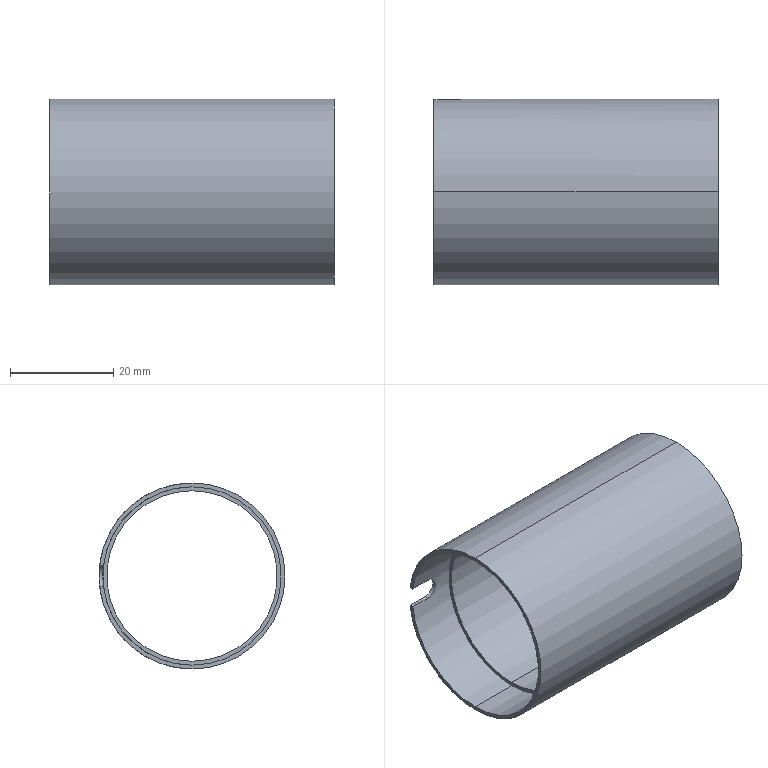Part | SolidWorks | features BaseBody 1 | 1 solid | 12 faces | box 55 x 36 x 36 mm | volume 8128 mm3 | cylinder 7 | plane 5 | commonest cylinder face diameters 33 x2 34.5 x2 36 x2 4.2 x1
STEP:
#1=CARTESIAN_POINT('',(-17.5,0.,16.5));
#2=VERTEX_POINT('',#1);
#3=CARTESIAN_POINT('',(-17.5,0.,-16.5));
#4=VERTEX_POINT('',#3);
#5=CARTESIAN_POINT('',(-17.5,0.,0.));
#6=DIRECTION('',(-1.,0.,0.));
#7=DIRECTION('',(0.,0.,1.));
#8=AXIS2_PLACEMENT_3D('',#5,#6,#7);
#9=CIRCLE('',#8,16.5);
#10=EDGE_CURVE('',#2,#4,#9,.T.);
#11=ORIENTED_EDGE('',*,*,#10,.F.);
#12=CARTESIAN_POINT('',(-17.5,0.,0.));
#13=DIRECTION('',(-1.,0.,0.));
#14=DIRECTION('',(0.,0.,1.));
#15=AXIS2_PLACEMENT_3D('',#12,#13,#14);
#16=CIRCLE('',#15,16.5);
#17=EDGE_CURVE('',#4,#2,#16,.T.);
#18=ORIENTED_EDGE('',*,*,#17,.F.);
#19=EDGE_LOOP('',(#11,#18));
#20=FACE_BOUND('',#19,.T.);
#21=CARTESIAN_POINT('',(-17.5,0.,17.25));
#22=VERTEX_POINT('',#21);
#23=CARTESIAN_POINT('',(-17.5,0.,-17.25));
#24=VERTEX_POINT('',#23);
#25=CARTESIAN_POINT('',(-17.5,0.,0.));
#26=DIRECTION('',(-1.,0.,0.));
#27=DIRECTION('',(0.,0.,1.));
#28=AXIS2_PLACEMENT_3D('',#25,#26,#27);
#29=CIRCLE('',#28,17.25);
#30=EDGE_CURVE('',#22,#24,#29,.T.);
#31=ORIENTED_EDGE('',*,*,#30,.T.);
#32=CARTESIAN_POINT('',(-17.5,0.,0.));
#33=DIRECTION('',(-1.,0.,0.));
#34=DIRECTION('',(0.,0.,1.));
#35=AXIS2_PLACEMENT_3D('',#32,#33,#34);
#36=CIRCLE('',#35,17.25);
#37=EDGE_CURVE('',#24,#22,#36,.T.);
#38=ORIENTED_EDGE('',*,*,#37,.T.);
#39=EDGE_LOOP('',(#31,#38));
#40=FACE_OUTER_BOUND('',#39,.T.);
#41=CARTESIAN_POINT('',(-17.5,0.,0.));
#42=DIRECTION('',(-1.,0.,0.));
#43=DIRECTION('',(0.,0.,1.));
#44=AXIS2_PLACEMENT_3D('',#41,#42,#43);
#45=PLANE('',#44);
#46=ADVANCED_FACE('',(#20,#40),#45,.T.);
#47=CARTESIAN_POINT('',(-27.5,0.,-17.25));
#48=VERTEX_POINT('',#47);
#49=CARTESIAN_POINT('',(-17.5,0.,-17.25));
#50=DIRECTION('',(-1.,0.,0.));
#51=VECTOR('',#50,1000.);
#52=LINE('',#49,#51);
#53=EDGE_CURVE('',#24,#48,#52,.T.);
#54=ORIENTED_EDGE('',*,*,#53,.F.);
#55=ORIENTED_EDGE('',*,*,#30,.F.);
#56=CARTESIAN_POINT('',(-27.5,0.,17.25));
#57=VERTEX_POINT('',#56);
#58=CARTESIAN_POINT('',(-17.5,0.,17.25));
#59=DIRECTION('',(-1.,0.,0.));
#60=VECTOR('',#59,1000.);
#61=LINE('',#58,#60);
#62=EDGE_CURVE('',#22,#57,#61,.T.);
#63=ORIENTED_EDGE('',*,*,#62,.T.);
#64=CARTESIAN_POINT('',(-27.5,17.122,2.1));
#65=VERTEX_POINT('',#64);
#66=CARTESIAN_POINT('',(-27.5,0.,0.));
#67=DIRECTION('',(-1.,0.,0.));
#68=DIRECTION('',(0.,0.,1.));
#69=AXIS2_PLACEMENT_3D('',#66,#67,#68);
#70=CIRCLE('',#69,17.25);
#71=EDGE_CURVE('',#57,#65,#70,.T.);
#72=ORIENTED_EDGE('',*,*,#71,.T.);
#73=CARTESIAN_POINT('',(-23.3,17.122,2.1));
#74=VERTEX_POINT('',#73);
#75=CARTESIAN_POINT('',(-17.5,17.122,2.1));
#76=DIRECTION('',(1.,0.,0.));
#77=VECTOR('',#76,1000.);
#78=LINE('',#75,#77);
#79=EDGE_CURVE('',#65,#74,#78,.T.);
#80=ORIENTED_EDGE('',*,*,#79,.T.);
#81=CARTESIAN_POINT('',(-23.3,17.122,-2.1));
#82=VERTEX_POINT('',#81);
#83=CARTESIAN_POINT('',(-23.3,17.122,2.1));
#84=CARTESIAN_POINT('',(-23.021,17.122,2.1));
#85=CARTESIAN_POINT('',(-22.752,17.129,2.046));
#86=CARTESIAN_POINT('',(-22.239,17.153,1.833));
#87=CARTESIAN_POINT('',(-22.012,17.169,1.681));
#88=CARTESIAN_POINT('',(-21.619,17.203,1.288));
#89=CARTESIAN_POINT('',(-21.467,17.219,1.062));
#90=CARTESIAN_POINT('',(-21.254,17.243,0.5477));
#91=CARTESIAN_POINT('',(-21.2,17.25,0.2799));
#92=CARTESIAN_POINT('',(-21.2,17.25,-0.2768));
#93=CARTESIAN_POINT('',(-21.253,17.243,-0.5451));
#94=CARTESIAN_POINT('',(-21.466,17.219,-1.06));
#95=CARTESIAN_POINT('',(-21.617,17.203,-1.287));
#96=CARTESIAN_POINT('',(-22.011,17.169,-1.681));
#97=CARTESIAN_POINT('',(-22.237,17.153,-1.833));
#98=CARTESIAN_POINT('',(-22.752,17.129,-2.046));
#99=CARTESIAN_POINT('',(-23.021,17.122,-2.1));
#100=CARTESIAN_POINT('',(-23.3,17.122,-2.1));
#101=B_SPLINE_CURVE_WITH_KNOTS('',3,(#83,#84,#85,#86,#87,#88,#89,#90,#91,#92,#93,#94,#95,#96,#97,#98,#99,#100),.UNSPECIFIED.,.F.,.F.,(4,2,2,2,2,2,2,2,4),(0.,0.125,0.25,0.375,0.5,0.625,0.75,0.875,1.),.UNSPECIFIED.);
#102=EDGE_CURVE('',#74,#82,#101,.T.);
#103=ORIENTED_EDGE('',*,*,#102,.T.);
#104=CARTESIAN_POINT('',(-27.5,17.122,-2.1));
#105=VERTEX_POINT('',#104);
#106=CARTESIAN_POINT('',(-17.5,17.122,-2.1));
#107=DIRECTION('',(-1.,0.,0.));
#108=VECTOR('',#107,1000.);
#109=LINE('',#106,#108);
#110=EDGE_CURVE('',#82,#105,#109,.T.);
#111=ORIENTED_EDGE('',*,*,#110,.T.);
#112=CARTESIAN_POINT('',(-27.5,0.,0.));
#113=DIRECTION('',(-1.,0.,0.));
#114=DIRECTION('',(0.,0.,1.));
#115=AXIS2_PLACEMENT_3D('',#112,#113,#114);
#116=CIRCLE('',#115,17.25);
#117=EDGE_CURVE('',#105,#48,#116,.T.);
#118=ORIENTED_EDGE('',*,*,#117,.T.);
#119=EDGE_LOOP('',(#54,#55,#63,#72,#80,#103,#111,#118));
#120=FACE_OUTER_BOUND('',#119,.T.);
#121=CARTESIAN_POINT('',(-17.5,0.,0.));
#122=DIRECTION('',(-1.,0.,0.));
#123=DIRECTION('',(0.,0.,1.));
#124=AXIS2_PLACEMENT_3D('',#121,#122,#123);
#125=CYLINDRICAL_SURFACE('',#124,17.25);
#126=ADVANCED_FACE('',(#120),#125,.F.);
#127=ORIENTED_EDGE('',*,*,#79,.F.);
#128=CARTESIAN_POINT('',(-27.5,17.877,2.1));
#129=VERTEX_POINT('',#128);
#130=CARTESIAN_POINT('',(-27.5,50.,2.1));
#131=DIRECTION('',(0.,-1.,0.));
#132=VECTOR('',#131,1000.);
#133=LINE('',#130,#132);
#134=EDGE_CURVE('',#129,#65,#133,.T.);
#135=ORIENTED_EDGE('',*,*,#134,.F.);
#136=CARTESIAN_POINT('',(-23.3,17.877,2.1));
#137=VERTEX_POINT('',#136);
#138=CARTESIAN_POINT('',(27.5,17.877,2.1));
#139=DIRECTION('',(1.,0.,0.));
#140=VECTOR('',#139,1000.);
#141=LINE('',#138,#140);
#142=EDGE_CURVE('',#129,#137,#141,.T.);
#143=ORIENTED_EDGE('',*,*,#142,.T.);
#144=CARTESIAN_POINT('',(-23.3,50.,2.1));
#145=DIRECTION('',(0.,-1.,0.));
#146=VECTOR('',#145,1000.);
#147=LINE('',#144,#146);
#148=EDGE_CURVE('',#137,#74,#147,.T.);
#149=ORIENTED_EDGE('',*,*,#148,.T.);
#150=EDGE_LOOP('',(#127,#135,#143,#149));
#151=FACE_OUTER_BOUND('',#150,.T.);
#152=CARTESIAN_POINT('',(-23.3,50.,2.1));
#153=DIRECTION('',(0.,0.,-1.));
#154=DIRECTION('',(-1.,0.,0.));
#155=AXIS2_PLACEMENT_3D('',#152,#153,#154);
#156=PLANE('',#155);
#157=ADVANCED_FACE('',(#151),#156,.T.);
#158=ORIENTED_EDGE('',*,*,#110,.F.);
#159=CARTESIAN_POINT('',(-23.3,17.877,-2.1));
#160=VERTEX_POINT('',#159);
#161=CARTESIAN_POINT('',(-23.3,50.,-2.1));
#162=DIRECTION('',(0.,-1.,0.));
#163=VECTOR('',#162,1000.);
#164=LINE('',#161,#163);
#165=EDGE_CURVE('',#160,#82,#164,.T.);
#166=ORIENTED_EDGE('',*,*,#165,.F.);
#167=CARTESIAN_POINT('',(-27.5,17.877,-2.1));
#168=VERTEX_POINT('',#167);
#169=CARTESIAN_POINT('',(27.5,17.877,-2.1));
#170=DIRECTION('',(-1.,0.,0.));
#171=VECTOR('',#170,1000.);
#172=LINE('',#169,#171);
#173=EDGE_CURVE('',#160,#168,#172,.T.);
#174=ORIENTED_EDGE('',*,*,#173,.T.);
#175=CARTESIAN_POINT('',(-27.5,50.,-2.1));
#176=DIRECTION('',(0.,-1.,0.));
#177=VECTOR('',#176,1000.);
#178=LINE('',#175,#177);
#179=EDGE_CURVE('',#168,#105,#178,.T.);
#180=ORIENTED_EDGE('',*,*,#179,.T.);
#181=EDGE_LOOP('',(#158,#166,#174,#180));
#182=FACE_OUTER_BOUND('',#181,.T.);
#183=CARTESIAN_POINT('',(-23.3,50.,-2.1));
#184=DIRECTION('',(0.,0.,1.));
#185=DIRECTION('',(1.,0.,0.));
#186=AXIS2_PLACEMENT_3D('',#183,#184,#185);
#187=PLANE('',#186);
#188=ADVANCED_FACE('',(#182),#187,.T.);
#189=ORIENTED_EDGE('',*,*,#102,.F.);
#190=ORIENTED_EDGE('',*,*,#148,.F.);
#191=CARTESIAN_POINT('',(-23.3,17.877,2.1));
#192=CARTESIAN_POINT('',(-23.17,17.877,2.1));
#193=CARTESIAN_POINT('',(-23.036,17.879,2.088));
#194=CARTESIAN_POINT('',(-22.834,17.883,2.049));
#195=CARTESIAN_POINT('',(-22.766,17.885,2.032));
#196=CARTESIAN_POINT('',(-22.664,17.888,2.002));
#197=CARTESIAN_POINT('',(-22.613,17.89,1.985));
#198=CARTESIAN_POINT('',(-22.554,17.893,1.963));
#199=CARTESIAN_POINT('',(-22.525,17.894,1.952));
#200=CARTESIAN_POINT('',(-22.512,17.894,1.947));
#201=CARTESIAN_POINT('',(-22.504,17.895,1.943));
#202=CARTESIAN_POINT('',(-22.498,17.895,1.941));
#203=CARTESIAN_POINT('',(-22.41,17.899,1.904));
#204=CARTESIAN_POINT('',(-22.305,17.905,1.855));
#205=CARTESIAN_POINT('',(-22.072,17.919,1.709));
#206=CARTESIAN_POINT('',(-21.943,17.928,1.613));
#207=CARTESIAN_POINT('',(-21.687,17.949,1.357));
#208=CARTESIAN_POINT('',(-21.592,17.958,1.229));
#209=CARTESIAN_POINT('',(-21.483,17.969,1.054));
#210=CARTESIAN_POINT('',(-21.452,17.972,0.999));
#211=CARTESIAN_POINT('',(-21.413,17.976,0.9217));
#212=CARTESIAN_POINT('',(-21.401,17.978,0.8968));
#213=CARTESIAN_POINT('',(-21.385,17.979,0.8611));
#214=CARTESIAN_POINT('',(-21.377,17.98,0.8436));
#215=CARTESIAN_POINT('',(-21.368,17.981,0.8239));
#216=CARTESIAN_POINT('',(-21.365,17.982,0.8156));
#217=CARTESIAN_POINT('',(-21.363,17.982,0.8102));
#218=CARTESIAN_POINT('',(-21.362,17.982,0.8089));
#219=CARTESIAN_POINT('',(-21.249,17.994,0.5371));
#220=CARTESIAN_POINT('',(-21.2,18.,0.2615));
#221=CARTESIAN_POINT('',(-21.2,18.,-0.1285));
#222=CARTESIAN_POINT('',(-21.212,17.999,-0.2623));
#223=CARTESIAN_POINT('',(-21.251,17.994,-0.4648));
#224=CARTESIAN_POINT('',(-21.267,17.992,-0.5325));
#225=CARTESIAN_POINT('',(-21.298,17.989,-0.634));
#226=CARTESIAN_POINT('',(-21.314,17.987,-0.6847));
#227=CARTESIAN_POINT('',(-21.336,17.985,-0.7436));
#228=CARTESIAN_POINT('',(-21.347,17.983,-0.773));
#229=CARTESIAN_POINT('',(-21.352,17.983,-0.7856));
#230=CARTESIAN_POINT('',(-21.356,17.982,-0.794));
#231=CARTESIAN_POINT('',(-21.358,17.982,-0.7996));
#232=CARTESIAN_POINT('',(-21.395,17.978,-0.8894));
#233=CARTESIAN_POINT('',(-21.445,17.973,-0.9943));
#234=CARTESIAN_POINT('',(-21.591,17.958,-1.228));
#235=CARTESIAN_POINT('',(-21.686,17.949,-1.355));
#236=CARTESIAN_POINT('',(-21.943,17.928,-1.613));
#237=CARTESIAN_POINT('',(-22.072,17.919,-1.709));
#238=CARTESIAN_POINT('',(-22.246,17.908,-1.818));
#239=CARTESIAN_POINT('',(-22.302,17.905,-1.848));
#240=CARTESIAN_POINT('',(-22.379,17.901,-1.887));
#241=CARTESIAN_POINT('',(-22.404,17.9,-1.899));
#242=CARTESIAN_POINT('',(-22.439,17.898,-1.915));
#243=CARTESIAN_POINT('',(-22.456,17.897,-1.923));
#244=CARTESIAN_POINT('',(-22.476,17.896,-1.932));
#245=CARTESIAN_POINT('',(-22.484,17.896,-1.935));
#246=CARTESIAN_POINT('',(-22.49,17.895,-1.937));
#247=CARTESIAN_POINT('',(-22.491,17.895,-1.938));
#248=CARTESIAN_POINT('',(-22.763,17.883,-2.051));
#249=CARTESIAN_POINT('',(-23.04,17.877,-2.1));
#250=CARTESIAN_POINT('',(-23.3,17.877,-2.1));
#251=B_SPLINE_CURVE_WITH_KNOTS('',3,(#191,#192,#193,#194,#195,#196,#197,#198,#199,#200,#201,#202,#203,#204,#205,#206,#207,#208,#209,#210,#211,#212,#213,#214,#215,#216,#217,#218,#219,#220,#221,#222,#223,#224,#225,#226,#227,#228,#229,#230,#231,#232,#233,#234,#235,#236,#237,#238,#239,#240,#241,#242,#243,#244,#245,#246,#247,#248,#249,#250),.UNSPECIFIED.,.F.,.F.,(4,2,2,1,1,1,2,2,2,2,2,2,2,1,1,2,2,2,2,2,1,1,1,2,2,2,2,2,2,2,1,1,2,2,4),(0.,0.0625,0.09375,0.1094,0.1172,0.1211,0.123,0.125,0.1875,0.25,0.3125,0.3437,0.3594,0.3672,0.3711,0.373,0.375,0.5,0.5625,0.5937,0.6094,0.6172,0.6211,0.623,0.625,0.6875,0.75,0.8125,0.8437,0.8594,0.8672,0.8711,0.873,0.875,1.),.UNSPECIFIED.);
#252=EDGE_CURVE('',#137,#160,#251,.T.);
#253=ORIENTED_EDGE('',*,*,#252,.T.);
#254=ORIENTED_EDGE('',*,*,#165,.T.);
#255=EDGE_LOOP('',(#189,#190,#253,#254));
#256=FACE_OUTER_BOUND('',#255,.T.);
#257=CARTESIAN_POINT('',(-23.3,50.,0.));
#258=DIRECTION('',(0.,-1.,0.));
#259=DIRECTION('',(0.,0.,-1.));
#260=AXIS2_PLACEMENT_3D('',#257,#258,#259);
#261=CYLINDRICAL_SURFACE('',#260,2.1);
#262=ADVANCED_FACE('',(#256),#261,.F.);
#263=CARTESIAN_POINT('',(27.5,0.,16.5));
#264=VERTEX_POINT('',#263);
#265=CARTESIAN_POINT('',(27.5,0.,-16.5));
#266=VERTEX_POINT('',#265);
#267=CARTESIAN_POINT('',(27.5,0.,0.));
#268=DIRECTION('',(1.,0.,0.));
#269=DIRECTION('',(0.,0.,-1.));
#270=AXIS2_PLACEMENT_3D('',#267,#268,#269);
#271=CIRCLE('',#270,16.5);
#272=EDGE_CURVE('',#264,#266,#271,.T.);
#273=ORIENTED_EDGE('',*,*,#272,.F.);
#274=CARTESIAN_POINT('',(27.5,0.,0.));
#275=DIRECTION('',(1.,0.,0.));
#276=DIRECTION('',(0.,0.,-1.));
#277=AXIS2_PLACEMENT_3D('',#274,#275,#276);
#278=CIRCLE('',#277,16.5);
#279=EDGE_CURVE('',#266,#264,#278,.T.);
#280=ORIENTED_EDGE('',*,*,#279,.F.);
#281=EDGE_LOOP('',(#273,#280));
#282=FACE_BOUND('',#281,.T.);
#283=CARTESIAN_POINT('',(27.5,0.,18.));
#284=VERTEX_POINT('',#283);
#285=CARTESIAN_POINT('',(27.5,0.,-18.));
#286=VERTEX_POINT('',#285);
#287=CARTESIAN_POINT('',(27.5,0.,0.));
#288=DIRECTION('',(1.,0.,0.));
#289=DIRECTION('',(0.,0.,-1.));
#290=AXIS2_PLACEMENT_3D('',#287,#288,#289);
#291=CIRCLE('',#290,18.);
#292=EDGE_CURVE('',#284,#286,#291,.T.);
#293=ORIENTED_EDGE('',*,*,#292,.T.);
#294=CARTESIAN_POINT('',(27.5,0.,0.));
#295=DIRECTION('',(1.,0.,0.));
#296=DIRECTION('',(0.,0.,-1.));
#297=AXIS2_PLACEMENT_3D('',#294,#295,#296);
#298=CIRCLE('',#297,18.);
#299=EDGE_CURVE('',#286,#284,#298,.T.);
#300=ORIENTED_EDGE('',*,*,#299,.T.);
#301=EDGE_LOOP('',(#293,#300));
#302=FACE_OUTER_BOUND('',#301,.T.);
#303=CARTESIAN_POINT('',(27.5,0.,0.));
#304=DIRECTION('',(1.,0.,0.));
#305=DIRECTION('',(0.,1.,0.));
#306=AXIS2_PLACEMENT_3D('',#303,#304,#305);
#307=PLANE('',#306);
#308=ADVANCED_FACE('',(#282,#302),#307,.T.);
#309=CARTESIAN_POINT('',(-27.5,0.,-18.));
#310=VERTEX_POINT('',#309);
#311=CARTESIAN_POINT('',(27.5,0.,-18.));
#312=DIRECTION('',(-1.,0.,0.));
#313=VECTOR('',#312,1000.);
#314=LINE('',#311,#313);
#315=EDGE_CURVE('',#286,#310,#314,.T.);
#316=ORIENTED_EDGE('',*,*,#315,.F.);
#317=ORIENTED_EDGE('',*,*,#292,.F.);
#318=CARTESIAN_POINT('',(-27.5,0.,18.));
#319=VERTEX_POINT('',#318);
#320=CARTESIAN_POINT('',(27.5,0.,18.));
#321=DIRECTION('',(-1.,0.,0.));
#322=VECTOR('',#321,1000.);
#323=LINE('',#320,#322);
#324=EDGE_CURVE('',#284,#319,#323,.T.);
#325=ORIENTED_EDGE('',*,*,#324,.T.);
#326=CARTESIAN_POINT('',(-27.5,0.,0.));
#327=DIRECTION('',(1.,0.,0.));
#328=DIRECTION('',(0.,0.,-1.));
#329=AXIS2_PLACEMENT_3D('',#326,#327,#328);
#330=CIRCLE('',#329,18.);
#331=EDGE_CURVE('',#319,#310,#330,.T.);
#332=ORIENTED_EDGE('',*,*,#331,.T.);
#333=EDGE_LOOP('',(#316,#317,#325,#332));
#334=FACE_OUTER_BOUND('',#333,.T.);
#335=CARTESIAN_POINT('',(27.5,0.,0.));
#336=DIRECTION('',(-1.,0.,0.));
#337=DIRECTION('',(0.,0.,1.));
#338=AXIS2_PLACEMENT_3D('',#335,#336,#337);
#339=CYLINDRICAL_SURFACE('',#338,18.);
#340=ADVANCED_FACE('',(#334),#339,.T.);
#341=ORIENTED_EDGE('',*,*,#134,.T.);
#342=ORIENTED_EDGE('',*,*,#71,.F.);
#343=CARTESIAN_POINT('',(-27.5,0.,0.));
#344=DIRECTION('',(-1.,0.,0.));
#345=DIRECTION('',(0.,0.,1.));
#346=AXIS2_PLACEMENT_3D('',#343,#344,#345);
#347=CIRCLE('',#346,17.25);
#348=EDGE_CURVE('',#48,#57,#347,.T.);
#349=ORIENTED_EDGE('',*,*,#348,.F.);
#350=ORIENTED_EDGE('',*,*,#117,.F.);
#351=ORIENTED_EDGE('',*,*,#179,.F.);
#352=CARTESIAN_POINT('',(-27.5,0.,0.));
#353=DIRECTION('',(1.,0.,0.));
#354=DIRECTION('',(0.,0.,-1.));
#355=AXIS2_PLACEMENT_3D('',#352,#353,#354);
#356=CIRCLE('',#355,18.);
#357=EDGE_CURVE('',#310,#168,#356,.T.);
#358=ORIENTED_EDGE('',*,*,#357,.F.);
#359=ORIENTED_EDGE('',*,*,#331,.F.);
#360=CARTESIAN_POINT('',(-27.5,0.,0.));
#361=DIRECTION('',(1.,0.,0.));
#362=DIRECTION('',(0.,0.,-1.));
#363=AXIS2_PLACEMENT_3D('',#360,#361,#362);
#364=CIRCLE('',#363,18.);
#365=EDGE_CURVE('',#129,#319,#364,.T.);
#366=ORIENTED_EDGE('',*,*,#365,.F.);
#367=EDGE_LOOP('',(#341,#342,#349,#350,#351,#358,#359,#366));
#368=FACE_OUTER_BOUND('',#367,.T.);
#369=CARTESIAN_POINT('',(-27.5,0.,0.));
#370=DIRECTION('',(1.,0.,0.));
#371=DIRECTION('',(0.,1.,0.));
#372=AXIS2_PLACEMENT_3D('',#369,#370,#371);
#373=PLANE('',#372);
#374=ADVANCED_FACE('',(#368),#373,.F.);
#375=CARTESIAN_POINT('',(27.5,0.,-16.5));
#376=DIRECTION('',(-1.,0.,0.));
#377=VECTOR('',#376,1000.);
#378=LINE('',#375,#377);
#379=EDGE_CURVE('',#266,#4,#378,.T.);
#380=ORIENTED_EDGE('',*,*,#379,.F.);
#381=ORIENTED_EDGE('',*,*,#279,.T.);
#382=CARTESIAN_POINT('',(27.5,0.,16.5));
#383=DIRECTION('',(-1.,0.,0.));
#384=VECTOR('',#383,1000.);
#385=LINE('',#382,#384);
#386=EDGE_CURVE('',#264,#2,#385,.T.);
#387=ORIENTED_EDGE('',*,*,#386,.T.);
#388=ORIENTED_EDGE('',*,*,#10,.T.);
#389=EDGE_LOOP('',(#380,#381,#387,#388));
#390=FACE_OUTER_BOUND('',#389,.T.);
#391=CARTESIAN_POINT('',(27.5,0.,0.));
#392=DIRECTION('',(-1.,0.,0.));
#393=DIRECTION('',(0.,0.,1.));
#394=AXIS2_PLACEMENT_3D('',#391,#392,#393);
#395=CYLINDRICAL_SURFACE('',#394,16.5);
#396=ADVANCED_FACE('',(#390),#395,.F.);
#397=ORIENTED_EDGE('',*,*,#272,.T.);
#398=ORIENTED_EDGE('',*,*,#379,.T.);
#399=ORIENTED_EDGE('',*,*,#17,.T.);
#400=ORIENTED_EDGE('',*,*,#386,.F.);
#401=EDGE_LOOP('',(#397,#398,#399,#400));
#402=FACE_OUTER_BOUND('',#401,.T.);
#403=CARTESIAN_POINT('',(27.5,0.,0.));
#404=DIRECTION('',(-1.,0.,0.));
#405=DIRECTION('',(0.,0.,1.));
#406=AXIS2_PLACEMENT_3D('',#403,#404,#405);
#407=CYLINDRICAL_SURFACE('',#406,16.5);
#408=ADVANCED_FACE('',(#402),#407,.F.);
#409=ORIENTED_EDGE('',*,*,#299,.F.);
#410=ORIENTED_EDGE('',*,*,#315,.T.);
#411=ORIENTED_EDGE('',*,*,#357,.T.);
#412=ORIENTED_EDGE('',*,*,#173,.F.);
#413=ORIENTED_EDGE('',*,*,#252,.F.);
#414=ORIENTED_EDGE('',*,*,#142,.F.);
#415=ORIENTED_EDGE('',*,*,#365,.T.);
#416=ORIENTED_EDGE('',*,*,#324,.F.);
#417=EDGE_LOOP('',(#409,#410,#411,#412,#413,#414,#415,#416));
#418=FACE_OUTER_BOUND('',#417,.T.);
#419=CARTESIAN_POINT('',(27.5,0.,0.));
#420=DIRECTION('',(-1.,0.,0.));
#421=DIRECTION('',(0.,0.,1.));
#422=AXIS2_PLACEMENT_3D('',#419,#420,#421);
#423=CYLINDRICAL_SURFACE('',#422,18.);
#424=ADVANCED_FACE('',(#418),#423,.T.);
#425=ORIENTED_EDGE('',*,*,#37,.F.);
#426=ORIENTED_EDGE('',*,*,#53,.T.);
#427=ORIENTED_EDGE('',*,*,#348,.T.);
#428=ORIENTED_EDGE('',*,*,#62,.F.);
#429=EDGE_LOOP('',(#425,#426,#427,#428));
#430=FACE_OUTER_BOUND('',#429,.T.);
#431=CARTESIAN_POINT('',(-17.5,0.,0.));
#432=DIRECTION('',(-1.,0.,0.));
#433=DIRECTION('',(0.,0.,1.));
#434=AXIS2_PLACEMENT_3D('',#431,#432,#433);
#435=CYLINDRICAL_SURFACE('',#434,17.25);
#436=ADVANCED_FACE('',(#430),#435,.F.);
#437=CLOSED_SHELL('',(#46,#126,#157,#188,#262,#308,#340,#374,#396,#408,#424,#436));
#438=MANIFOLD_SOLID_BREP('',#437);
#439=CARTESIAN_POINT('',(0.,0.,0.));
#440=DIRECTION('',(0.,0.,1.));
#441=DIRECTION('',(1.,0.,0.));
#442=AXIS2_PLACEMENT_3D('',#439,#440,#441);
#443=(LENGTH_UNIT()NAMED_UNIT(*)SI_UNIT(.MILLI.,.METRE.));
#444=UNCERTAINTY_MEASURE_WITH_UNIT(LENGTH_MEASURE(0.00001),#443,'','');
#445=(NAMED_UNIT(*)PLANE_ANGLE_UNIT()SI_UNIT($,.RADIAN.));
#446=(NAMED_UNIT(*)SI_UNIT($,.STERADIAN.)SOLID_ANGLE_UNIT());
#447=(GEOMETRIC_REPRESENTATION_CONTEXT(3)GLOBAL_UNCERTAINTY_ASSIGNED_CONTEXT((#444))GLOBAL_UNIT_ASSIGNED_CONTEXT((#443,#445,#446))REPRESENTATION_CONTEXT('',''));
#448=ADVANCED_BREP_SHAPE_REPRESENTATION('',(#438,#442),#447);